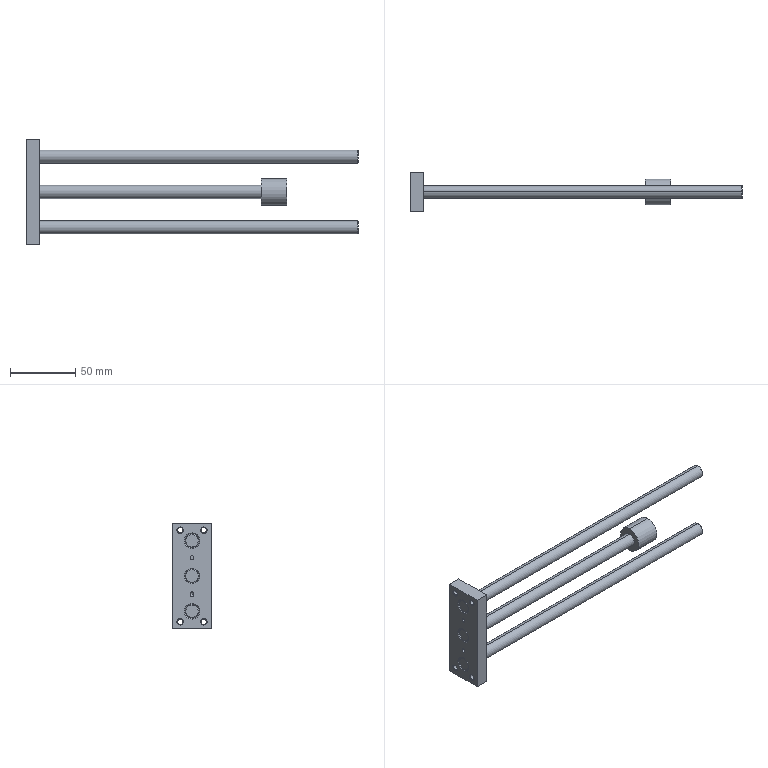Part | SolidWorks | features BaseBody 1 | 1 solid | 90 faces | box 254 x 30 x 81 mm | volume 81156 mm3 | cylinder 35 | cone 34 | plane 21 | commonest cylinder face diameters 4.134 x8 3 x7 10 x6 10.5 x6 11 x6 19.9 x2